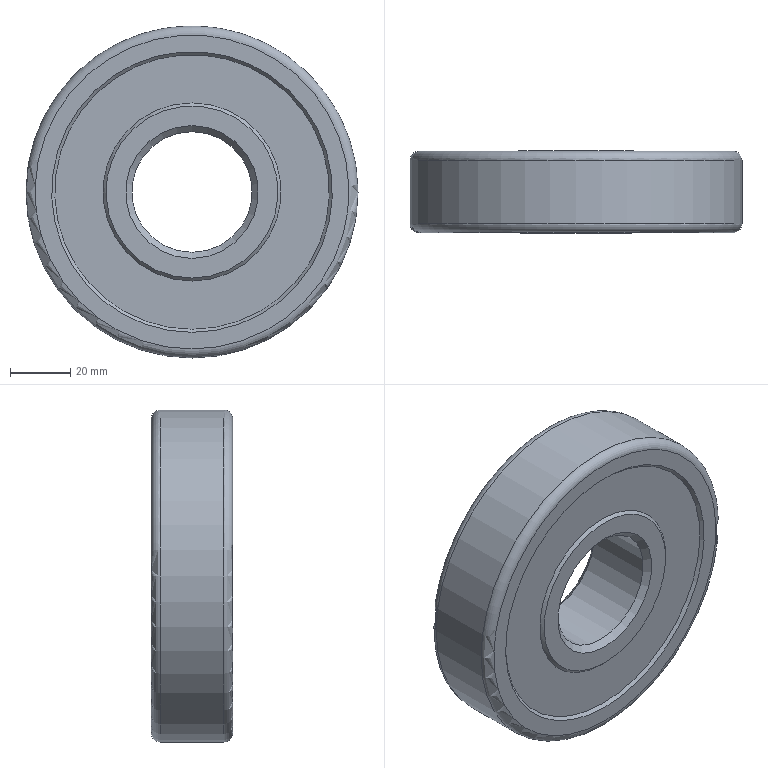Part | NX | features BREP 1, DATUM_CSYS 1 | 1 solid | 24 faces | box 110 x 27 x 110 mm | volume 123017 mm3 | plane 8 | cone 6 | cylinder 6 | torus 4 | commonest cylinder face diameters 61 x2 89 x2 40 x1 110 x1
STEP:
#1=CARTESIAN_POINT('',(0.,638.,-22.));
#2=VERTEX_POINT('',#1);
#3=CARTESIAN_POINT('',(0.,638.,0.));
#4=DIRECTION('',(0.,-1.,0.));
#5=DIRECTION('',(0.,0.,-1.));
#6=AXIS2_PLACEMENT_3D('',#3,#4,#5);
#7=CIRCLE('',#6,22.);
#8=EDGE_CURVE('',#2,#2,#7,.F.);
#9=ORIENTED_EDGE('',*,*,#8,.T.);
#10=EDGE_LOOP('',(#9));
#11=FACE_BOUND('',#10,.T.);
#12=CARTESIAN_POINT('',(0.,636.,-20.));
#13=VERTEX_POINT('',#12);
#14=CARTESIAN_POINT('',(0.,636.,0.));
#15=DIRECTION('',(0.,-1.,0.));
#16=DIRECTION('',(0.,0.,-1.));
#17=AXIS2_PLACEMENT_3D('',#14,#15,#16);
#18=CIRCLE('',#17,20.);
#19=EDGE_CURVE('',#13,#13,#18,.F.);
#20=ORIENTED_EDGE('',*,*,#19,.F.);
#21=EDGE_LOOP('',(#20));
#22=FACE_BOUND('',#21,.T.);
#23=CARTESIAN_POINT('',(0.,636.,0.));
#24=DIRECTION('',(0.,1.,0.));
#25=DIRECTION('',(0.,0.,-1.));
#26=AXIS2_PLACEMENT_3D('',#23,#24,#25);
#27=CONICAL_SURFACE('',#26,20.,0.7854);
#28=ADVANCED_FACE('',(#11,#22),#27,.F.);
#29=CARTESIAN_POINT('',(0.,638.,-28.5));
#30=VERTEX_POINT('',#29);
#31=CARTESIAN_POINT('',(0.,638.,0.));
#32=DIRECTION('',(0.,-1.,0.));
#33=DIRECTION('',(0.,0.,-1.));
#34=AXIS2_PLACEMENT_3D('',#31,#32,#33);
#35=CIRCLE('',#34,28.5);
#36=EDGE_CURVE('',#30,#30,#35,.F.);
#37=ORIENTED_EDGE('',*,*,#36,.T.);
#38=EDGE_LOOP('',(#37));
#39=FACE_BOUND('',#38,.T.);
#40=ORIENTED_EDGE('',*,*,#8,.F.);
#41=EDGE_LOOP('',(#40));
#42=FACE_BOUND('',#41,.T.);
#43=CARTESIAN_POINT('',(22.,638.,0.));
#44=DIRECTION('',(0.,1.,0.));
#45=DIRECTION('',(0.,0.,-1.));
#46=AXIS2_PLACEMENT_3D('',#43,#44,#45);
#47=PLANE('',#46);
#48=ADVANCED_FACE('',(#39,#42),#47,.T.);
#49=CARTESIAN_POINT('',(0.,637.,-29.5));
#50=VERTEX_POINT('',#49);
#51=CARTESIAN_POINT('',(0.,637.,0.));
#52=DIRECTION('',(0.,-1.,0.));
#53=DIRECTION('',(0.,0.,-1.));
#54=AXIS2_PLACEMENT_3D('',#51,#52,#53);
#55=CIRCLE('',#54,29.5);
#56=EDGE_CURVE('',#50,#50,#55,.F.);
#57=ORIENTED_EDGE('',*,*,#56,.T.);
#58=EDGE_LOOP('',(#57));
#59=FACE_BOUND('',#58,.T.);
#60=ORIENTED_EDGE('',*,*,#36,.F.);
#61=EDGE_LOOP('',(#60));
#62=FACE_BOUND('',#61,.T.);
#63=CARTESIAN_POINT('',(0.,638.,0.));
#64=DIRECTION('',(0.,-1.,0.));
#65=DIRECTION('',(0.,0.,1.));
#66=AXIS2_PLACEMENT_3D('',#63,#64,#65);
#67=CONICAL_SURFACE('',#66,28.5,0.7854);
#68=ADVANCED_FACE('',(#59,#62),#67,.T.);
#69=CARTESIAN_POINT('',(0.,637.,-45.5));
#70=VERTEX_POINT('',#69);
#71=CARTESIAN_POINT('',(0.,637.,0.));
#72=DIRECTION('',(0.,-1.,0.));
#73=DIRECTION('',(0.,0.,-1.));
#74=AXIS2_PLACEMENT_3D('',#71,#72,#73);
#75=CIRCLE('',#74,45.5);
#76=EDGE_CURVE('',#70,#70,#75,.F.);
#77=ORIENTED_EDGE('',*,*,#76,.T.);
#78=EDGE_LOOP('',(#77));
#79=FACE_BOUND('',#78,.T.);
#80=ORIENTED_EDGE('',*,*,#56,.F.);
#81=EDGE_LOOP('',(#80));
#82=FACE_BOUND('',#81,.T.);
#83=CARTESIAN_POINT('',(29.5,637.,0.));
#84=DIRECTION('',(0.,1.,0.));
#85=DIRECTION('',(0.,0.,-1.));
#86=AXIS2_PLACEMENT_3D('',#83,#84,#85);
#87=PLANE('',#86);
#88=ADVANCED_FACE('',(#79,#82),#87,.T.);
#89=CARTESIAN_POINT('',(0.,638.,-46.5));
#90=VERTEX_POINT('',#89);
#91=CARTESIAN_POINT('',(0.,638.,0.));
#92=DIRECTION('',(0.,-1.,0.));
#93=DIRECTION('',(0.,0.,-1.));
#94=AXIS2_PLACEMENT_3D('',#91,#92,#93);
#95=CIRCLE('',#94,46.5);
#96=EDGE_CURVE('',#90,#90,#95,.F.);
#97=ORIENTED_EDGE('',*,*,#96,.T.);
#98=EDGE_LOOP('',(#97));
#99=FACE_BOUND('',#98,.T.);
#100=ORIENTED_EDGE('',*,*,#76,.F.);
#101=EDGE_LOOP('',(#100));
#102=FACE_BOUND('',#101,.T.);
#103=CARTESIAN_POINT('',(0.,637.,0.));
#104=DIRECTION('',(0.,1.,0.));
#105=DIRECTION('',(0.,0.,-1.));
#106=AXIS2_PLACEMENT_3D('',#103,#104,#105);
#107=CONICAL_SURFACE('',#106,45.5,0.7854);
#108=ADVANCED_FACE('',(#99,#102),#107,.F.);
#109=CARTESIAN_POINT('',(0.,638.,-52.));
#110=VERTEX_POINT('',#109);
#111=CARTESIAN_POINT('',(0.,638.,0.));
#112=DIRECTION('',(0.,-1.,0.));
#113=DIRECTION('',(0.,0.,-1.));
#114=AXIS2_PLACEMENT_3D('',#111,#112,#113);
#115=CIRCLE('',#114,52.);
#116=EDGE_CURVE('',#110,#110,#115,.F.);
#117=ORIENTED_EDGE('',*,*,#116,.T.);
#118=EDGE_LOOP('',(#117));
#119=FACE_BOUND('',#118,.T.);
#120=ORIENTED_EDGE('',*,*,#96,.F.);
#121=EDGE_LOOP('',(#120));
#122=FACE_BOUND('',#121,.T.);
#123=CARTESIAN_POINT('',(46.5,638.,0.));
#124=DIRECTION('',(0.,1.,0.));
#125=DIRECTION('',(0.,0.,-1.));
#126=AXIS2_PLACEMENT_3D('',#123,#124,#125);
#127=PLANE('',#126);
#128=ADVANCED_FACE('',(#119,#122),#127,.T.);
#129=CARTESIAN_POINT('',(0.,635.,-55.));
#130=VERTEX_POINT('',#129);
#131=CARTESIAN_POINT('',(0.,635.,0.));
#132=DIRECTION('',(0.,-1.,0.));
#133=DIRECTION('',(0.,0.,-1.));
#134=AXIS2_PLACEMENT_3D('',#131,#132,#133);
#135=CIRCLE('',#134,55.);
#136=EDGE_CURVE('',#130,#130,#135,.F.);
#137=ORIENTED_EDGE('',*,*,#136,.T.);
#138=EDGE_LOOP('',(#137));
#139=FACE_BOUND('',#138,.T.);
#140=ORIENTED_EDGE('',*,*,#116,.F.);
#141=EDGE_LOOP('',(#140));
#142=FACE_BOUND('',#141,.T.);
#143=CARTESIAN_POINT('',(0.,635.,0.));
#144=DIRECTION('',(0.,1.,0.));
#145=DIRECTION('',(0.,0.,-1.));
#146=AXIS2_PLACEMENT_3D('',#143,#144,#145);
#147=TOROIDAL_SURFACE('',#146,52.,3.);
#148=ADVANCED_FACE('',(#139,#142),#147,.T.);
#149=CARTESIAN_POINT('',(0.,614.,-55.));
#150=VERTEX_POINT('',#149);
#151=CARTESIAN_POINT('',(0.,614.,0.));
#152=DIRECTION('',(0.,-1.,0.));
#153=DIRECTION('',(0.,0.,-1.));
#154=AXIS2_PLACEMENT_3D('',#151,#152,#153);
#155=CIRCLE('',#154,55.);
#156=EDGE_CURVE('',#150,#150,#155,.F.);
#157=ORIENTED_EDGE('',*,*,#156,.T.);
#158=EDGE_LOOP('',(#157));
#159=FACE_BOUND('',#158,.T.);
#160=ORIENTED_EDGE('',*,*,#136,.F.);
#161=EDGE_LOOP('',(#160));
#162=FACE_BOUND('',#161,.T.);
#163=CARTESIAN_POINT('',(0.,611.,0.));
#164=DIRECTION('',(0.,1.,0.));
#165=DIRECTION('',(0.,0.,-1.));
#166=AXIS2_PLACEMENT_3D('',#163,#164,#165);
#167=CYLINDRICAL_SURFACE('',#166,55.);
#168=ADVANCED_FACE('',(#159,#162),#167,.T.);
#169=CARTESIAN_POINT('',(0.,611.,-52.));
#170=VERTEX_POINT('',#169);
#171=CARTESIAN_POINT('',(0.,611.,0.));
#172=DIRECTION('',(0.,-1.,0.));
#173=DIRECTION('',(0.,0.,-1.));
#174=AXIS2_PLACEMENT_3D('',#171,#172,#173);
#175=CIRCLE('',#174,52.);
#176=EDGE_CURVE('',#170,#170,#175,.F.);
#177=ORIENTED_EDGE('',*,*,#176,.T.);
#178=EDGE_LOOP('',(#177));
#179=FACE_BOUND('',#178,.T.);
#180=ORIENTED_EDGE('',*,*,#156,.F.);
#181=EDGE_LOOP('',(#180));
#182=FACE_BOUND('',#181,.T.);
#183=CARTESIAN_POINT('',(0.,614.,0.));
#184=DIRECTION('',(0.,1.,0.));
#185=DIRECTION('',(0.,0.,-1.));
#186=AXIS2_PLACEMENT_3D('',#183,#184,#185);
#187=TOROIDAL_SURFACE('',#186,52.,3.);
#188=ADVANCED_FACE('',(#179,#182),#187,.T.);
#189=CARTESIAN_POINT('',(0.,611.,-46.5));
#190=VERTEX_POINT('',#189);
#191=CARTESIAN_POINT('',(0.,611.,0.));
#192=DIRECTION('',(0.,-1.,0.));
#193=DIRECTION('',(0.,0.,-1.));
#194=AXIS2_PLACEMENT_3D('',#191,#192,#193);
#195=CIRCLE('',#194,46.5);
#196=EDGE_CURVE('',#190,#190,#195,.F.);
#197=ORIENTED_EDGE('',*,*,#196,.T.);
#198=EDGE_LOOP('',(#197));
#199=FACE_BOUND('',#198,.T.);
#200=ORIENTED_EDGE('',*,*,#176,.F.);
#201=EDGE_LOOP('',(#200));
#202=FACE_BOUND('',#201,.T.);
#203=CARTESIAN_POINT('',(52.,611.,0.));
#204=DIRECTION('',(0.,-1.,0.));
#205=DIRECTION('',(0.,0.,1.));
#206=AXIS2_PLACEMENT_3D('',#203,#204,#205);
#207=PLANE('',#206);
#208=ADVANCED_FACE('',(#199,#202),#207,.T.);
#209=CARTESIAN_POINT('',(0.,612.,-45.5));
#210=VERTEX_POINT('',#209);
#211=CARTESIAN_POINT('',(0.,612.,0.));
#212=DIRECTION('',(0.,-1.,0.));
#213=DIRECTION('',(0.,0.,-1.));
#214=AXIS2_PLACEMENT_3D('',#211,#212,#213);
#215=CIRCLE('',#214,45.5);
#216=EDGE_CURVE('',#210,#210,#215,.F.);
#217=ORIENTED_EDGE('',*,*,#216,.T.);
#218=EDGE_LOOP('',(#217));
#219=FACE_BOUND('',#218,.T.);
#220=ORIENTED_EDGE('',*,*,#196,.F.);
#221=EDGE_LOOP('',(#220));
#222=FACE_BOUND('',#221,.T.);
#223=CARTESIAN_POINT('',(0.,611.,0.));
#224=DIRECTION('',(0.,-1.,0.));
#225=DIRECTION('',(0.,0.,1.));
#226=AXIS2_PLACEMENT_3D('',#223,#224,#225);
#227=CONICAL_SURFACE('',#226,46.5,0.7854);
#228=ADVANCED_FACE('',(#219,#222),#227,.F.);
#229=CARTESIAN_POINT('',(0.,612.,-29.5));
#230=VERTEX_POINT('',#229);
#231=CARTESIAN_POINT('',(0.,612.,0.));
#232=DIRECTION('',(0.,-1.,0.));
#233=DIRECTION('',(0.,0.,-1.));
#234=AXIS2_PLACEMENT_3D('',#231,#232,#233);
#235=CIRCLE('',#234,29.5);
#236=EDGE_CURVE('',#230,#230,#235,.F.);
#237=ORIENTED_EDGE('',*,*,#236,.T.);
#238=EDGE_LOOP('',(#237));
#239=FACE_BOUND('',#238,.T.);
#240=ORIENTED_EDGE('',*,*,#216,.F.);
#241=EDGE_LOOP('',(#240));
#242=FACE_BOUND('',#241,.T.);
#243=CARTESIAN_POINT('',(45.5,612.,0.));
#244=DIRECTION('',(0.,-1.,0.));
#245=DIRECTION('',(0.,0.,1.));
#246=AXIS2_PLACEMENT_3D('',#243,#244,#245);
#247=PLANE('',#246);
#248=ADVANCED_FACE('',(#239,#242),#247,.T.);
#249=CARTESIAN_POINT('',(0.,611.,-28.5));
#250=VERTEX_POINT('',#249);
#251=CARTESIAN_POINT('',(0.,611.,0.));
#252=DIRECTION('',(0.,-1.,0.));
#253=DIRECTION('',(0.,0.,-1.));
#254=AXIS2_PLACEMENT_3D('',#251,#252,#253);
#255=CIRCLE('',#254,28.5);
#256=EDGE_CURVE('',#250,#250,#255,.F.);
#257=ORIENTED_EDGE('',*,*,#256,.T.);
#258=EDGE_LOOP('',(#257));
#259=FACE_BOUND('',#258,.T.);
#260=ORIENTED_EDGE('',*,*,#236,.F.);
#261=EDGE_LOOP('',(#260));
#262=FACE_BOUND('',#261,.T.);
#263=CARTESIAN_POINT('',(0.,612.,0.));
#264=DIRECTION('',(0.,1.,0.));
#265=DIRECTION('',(0.,0.,-1.));
#266=AXIS2_PLACEMENT_3D('',#263,#264,#265);
#267=CONICAL_SURFACE('',#266,29.5,0.7854);
#268=ADVANCED_FACE('',(#259,#262),#267,.T.);
#269=CARTESIAN_POINT('',(0.,611.,-22.));
#270=VERTEX_POINT('',#269);
#271=CARTESIAN_POINT('',(0.,611.,0.));
#272=DIRECTION('',(0.,-1.,0.));
#273=DIRECTION('',(0.,0.,-1.));
#274=AXIS2_PLACEMENT_3D('',#271,#272,#273);
#275=CIRCLE('',#274,22.);
#276=EDGE_CURVE('',#270,#270,#275,.F.);
#277=ORIENTED_EDGE('',*,*,#276,.T.);
#278=EDGE_LOOP('',(#277));
#279=FACE_BOUND('',#278,.T.);
#280=ORIENTED_EDGE('',*,*,#256,.F.);
#281=EDGE_LOOP('',(#280));
#282=FACE_BOUND('',#281,.T.);
#283=CARTESIAN_POINT('',(28.5,611.,0.));
#284=DIRECTION('',(0.,-1.,0.));
#285=DIRECTION('',(0.,0.,1.));
#286=AXIS2_PLACEMENT_3D('',#283,#284,#285);
#287=PLANE('',#286);
#288=ADVANCED_FACE('',(#279,#282),#287,.T.);
#289=CARTESIAN_POINT('',(0.,613.,-20.));
#290=VERTEX_POINT('',#289);
#291=CARTESIAN_POINT('',(0.,613.,0.));
#292=DIRECTION('',(0.,-1.,0.));
#293=DIRECTION('',(0.,0.,-1.));
#294=AXIS2_PLACEMENT_3D('',#291,#292,#293);
#295=CIRCLE('',#294,20.);
#296=EDGE_CURVE('',#290,#290,#295,.F.);
#297=ORIENTED_EDGE('',*,*,#296,.T.);
#298=EDGE_LOOP('',(#297));
#299=FACE_BOUND('',#298,.T.);
#300=ORIENTED_EDGE('',*,*,#276,.F.);
#301=EDGE_LOOP('',(#300));
#302=FACE_BOUND('',#301,.T.);
#303=CARTESIAN_POINT('',(0.,611.,0.));
#304=DIRECTION('',(0.,-1.,0.));
#305=DIRECTION('',(0.,0.,1.));
#306=AXIS2_PLACEMENT_3D('',#303,#304,#305);
#307=CONICAL_SURFACE('',#306,22.,0.7854);
#308=ADVANCED_FACE('',(#299,#302),#307,.F.);
#309=ORIENTED_EDGE('',*,*,#19,.T.);
#310=EDGE_LOOP('',(#309));
#311=FACE_BOUND('',#310,.T.);
#312=ORIENTED_EDGE('',*,*,#296,.F.);
#313=EDGE_LOOP('',(#312));
#314=FACE_BOUND('',#313,.T.);
#315=CARTESIAN_POINT('',(0.,611.,0.));
#316=DIRECTION('',(0.,1.,0.));
#317=DIRECTION('',(0.,0.,-1.));
#318=AXIS2_PLACEMENT_3D('',#315,#316,#317);
#319=CYLINDRICAL_SURFACE('',#318,20.);
#320=ADVANCED_FACE('',(#311,#314),#319,.F.);
#321=CLOSED_SHELL('',(#28,#48,#68,#88,#108,#128,#148,#168,#188,#208,#228,#248,#268,#288,#308,#320));
#322=CARTESIAN_POINT('',(0.,617.359,-30.5));
#323=VERTEX_POINT('',#322);
#324=CARTESIAN_POINT('',(0.,617.359,0.));
#325=DIRECTION('',(0.,-1.,0.));
#326=DIRECTION('',(0.,0.,-1.));
#327=AXIS2_PLACEMENT_3D('',#324,#325,#326);
#328=CIRCLE('',#327,30.5);
#329=EDGE_CURVE('',#323,#323,#328,.F.);
#330=ORIENTED_EDGE('',*,*,#329,.T.);
#331=EDGE_LOOP('',(#330));
#332=FACE_BOUND('',#331,.T.);
#333=CARTESIAN_POINT('',(0.,631.641,-30.5));
#334=VERTEX_POINT('',#333);
#335=CARTESIAN_POINT('',(0.,631.641,0.));
#336=DIRECTION('',(0.,-1.,0.));
#337=DIRECTION('',(0.,0.,-1.));
#338=AXIS2_PLACEMENT_3D('',#335,#336,#337);
#339=CIRCLE('',#338,30.5);
#340=EDGE_CURVE('',#334,#334,#339,.F.);
#341=ORIENTED_EDGE('',*,*,#340,.F.);
#342=EDGE_LOOP('',(#341));
#343=FACE_BOUND('',#342,.T.);
#344=CARTESIAN_POINT('',(0.,624.5,0.));
#345=DIRECTION('',(0.,1.,0.));
#346=DIRECTION('',(0.,0.,-1.));
#347=AXIS2_PLACEMENT_3D('',#344,#345,#346);
#348=TOROIDAL_SURFACE('',#347,37.5,10.);
#349=ADVANCED_FACE('',(#332,#343),#348,.F.);
#350=CARTESIAN_POINT('',(0.,613.,-30.5));
#351=VERTEX_POINT('',#350);
#352=CARTESIAN_POINT('',(0.,613.,0.));
#353=DIRECTION('',(0.,-1.,0.));
#354=DIRECTION('',(0.,0.,-1.));
#355=AXIS2_PLACEMENT_3D('',#352,#353,#354);
#356=CIRCLE('',#355,30.5);
#357=EDGE_CURVE('',#351,#351,#356,.F.);
#358=ORIENTED_EDGE('',*,*,#357,.T.);
#359=EDGE_LOOP('',(#358));
#360=FACE_BOUND('',#359,.T.);
#361=ORIENTED_EDGE('',*,*,#329,.F.);
#362=EDGE_LOOP('',(#361));
#363=FACE_BOUND('',#362,.T.);
#364=CARTESIAN_POINT('',(0.,611.,0.));
#365=DIRECTION('',(0.,1.,0.));
#366=DIRECTION('',(0.,0.,-1.));
#367=AXIS2_PLACEMENT_3D('',#364,#365,#366);
#368=CYLINDRICAL_SURFACE('',#367,30.5);
#369=ADVANCED_FACE('',(#360,#363),#368,.T.);
#370=CARTESIAN_POINT('',(0.,613.,-44.5));
#371=VERTEX_POINT('',#370);
#372=CARTESIAN_POINT('',(0.,613.,0.));
#373=DIRECTION('',(0.,-1.,0.));
#374=DIRECTION('',(0.,0.,-1.));
#375=AXIS2_PLACEMENT_3D('',#372,#373,#374);
#376=CIRCLE('',#375,44.5);
#377=EDGE_CURVE('',#371,#371,#376,.F.);
#378=ORIENTED_EDGE('',*,*,#377,.T.);
#379=EDGE_LOOP('',(#378));
#380=FACE_BOUND('',#379,.T.);
#381=ORIENTED_EDGE('',*,*,#357,.F.);
#382=EDGE_LOOP('',(#381));
#383=FACE_BOUND('',#382,.T.);
#384=CARTESIAN_POINT('',(30.5,613.,0.));
#385=DIRECTION('',(0.,1.,0.));
#386=DIRECTION('',(0.,0.,-1.));
#387=AXIS2_PLACEMENT_3D('',#384,#385,#386);
#388=PLANE('',#387);
#389=ADVANCED_FACE('',(#380,#383),#388,.T.);
#390=CARTESIAN_POINT('',(0.,617.359,-44.5));
#391=VERTEX_POINT('',#390);
#392=CARTESIAN_POINT('',(0.,617.359,0.));
#393=DIRECTION('',(0.,-1.,0.));
#394=DIRECTION('',(0.,0.,-1.));
#395=AXIS2_PLACEMENT_3D('',#392,#393,#394);
#396=CIRCLE('',#395,44.5);
#397=EDGE_CURVE('',#391,#391,#396,.F.);
#398=ORIENTED_EDGE('',*,*,#397,.T.);
#399=EDGE_LOOP('',(#398));
#400=FACE_BOUND('',#399,.T.);
#401=ORIENTED_EDGE('',*,*,#377,.F.);
#402=EDGE_LOOP('',(#401));
#403=FACE_BOUND('',#402,.T.);
#404=CARTESIAN_POINT('',(0.,611.,0.));
#405=DIRECTION('',(0.,1.,0.));
#406=DIRECTION('',(0.,0.,-1.));
#407=AXIS2_PLACEMENT_3D('',#404,#405,#406);
#408=CYLINDRICAL_SURFACE('',#407,44.5);
#409=ADVANCED_FACE('',(#400,#403),#408,.F.);
#410=CARTESIAN_POINT('',(0.,631.641,-44.5));
#411=VERTEX_POINT('',#410);
#412=CARTESIAN_POINT('',(0.,631.641,0.));
#413=DIRECTION('',(0.,-1.,0.));
#414=DIRECTION('',(0.,0.,-1.));
#415=AXIS2_PLACEMENT_3D('',#412,#413,#414);
#416=CIRCLE('',#415,44.5);
#417=EDGE_CURVE('',#411,#411,#416,.F.);
#418=ORIENTED_EDGE('',*,*,#417,.T.);
#419=EDGE_LOOP('',(#418));
#420=FACE_BOUND('',#419,.T.);
#421=ORIENTED_EDGE('',*,*,#397,.F.);
#422=EDGE_LOOP('',(#421));
#423=FACE_BOUND('',#422,.T.);
#424=CARTESIAN_POINT('',(0.,624.5,0.));
#425=DIRECTION('',(0.,1.,0.));
#426=DIRECTION('',(0.,0.,-1.));
#427=AXIS2_PLACEMENT_3D('',#424,#425,#426);
#428=TOROIDAL_SURFACE('',#427,37.5,10.);
#429=ADVANCED_FACE('',(#420,#423),#428,.F.);
#430=CARTESIAN_POINT('',(0.,636.,-44.5));
#431=VERTEX_POINT('',#430);
#432=CARTESIAN_POINT('',(0.,636.,0.));
#433=DIRECTION('',(0.,-1.,0.));
#434=DIRECTION('',(0.,0.,-1.));
#435=AXIS2_PLACEMENT_3D('',#432,#433,#434);
#436=CIRCLE('',#435,44.5);
#437=EDGE_CURVE('',#431,#431,#436,.F.);
#438=ORIENTED_EDGE('',*,*,#437,.T.);
#439=EDGE_LOOP('',(#438));
#440=FACE_BOUND('',#439,.T.);
#441=ORIENTED_EDGE('',*,*,#417,.F.);
#442=EDGE_LOOP('',(#441));
#443=FACE_BOUND('',#442,.T.);
#444=CARTESIAN_POINT('',(0.,611.,0.));
#445=DIRECTION('',(0.,1.,0.));
#446=DIRECTION('',(0.,0.,-1.));
#447=AXIS2_PLACEMENT_3D('',#444,#445,#446);
#448=CYLINDRICAL_SURFACE('',#447,44.5);
#449=ADVANCED_FACE('',(#440,#443),#448,.F.);
#450=CARTESIAN_POINT('',(0.,636.,-30.5));
#451=VERTEX_POINT('',#450);
#452=CARTESIAN_POINT('',(0.,636.,0.));
#453=DIRECTION('',(0.,-1.,0.));
#454=DIRECTION('',(0.,0.,-1.));
#455=AXIS2_PLACEMENT_3D('',#452,#453,#454);
#456=CIRCLE('',#455,30.5);
#457=EDGE_CURVE('',#451,#451,#456,.F.);
#458=ORIENTED_EDGE('',*,*,#457,.T.);
#459=EDGE_LOOP('',(#458));
#460=FACE_BOUND('',#459,.T.);
#461=ORIENTED_EDGE('',*,*,#437,.F.);
#462=EDGE_LOOP('',(#461));
#463=FACE_BOUND('',#462,.T.);
#464=CARTESIAN_POINT('',(44.5,636.,0.));
#465=DIRECTION('',(0.,-1.,0.));
#466=DIRECTION('',(0.,0.,1.));
#467=AXIS2_PLACEMENT_3D('',#464,#465,#466);
#468=PLANE('',#467);
#469=ADVANCED_FACE('',(#460,#463),#468,.T.);
#470=ORIENTED_EDGE('',*,*,#340,.T.);
#471=EDGE_LOOP('',(#470));
#472=FACE_BOUND('',#471,.T.);
#473=ORIENTED_EDGE('',*,*,#457,.F.);
#474=EDGE_LOOP('',(#473));
#475=FACE_BOUND('',#474,.T.);
#476=CARTESIAN_POINT('',(0.,611.,0.));
#477=DIRECTION('',(0.,1.,0.));
#478=DIRECTION('',(0.,0.,-1.));
#479=AXIS2_PLACEMENT_3D('',#476,#477,#478);
#480=CYLINDRICAL_SURFACE('',#479,30.5);
#481=ADVANCED_FACE('',(#472,#475),#480,.T.);
#482=CLOSED_SHELL('',(#349,#369,#389,#409,#429,#449,#469,#481));
#483=ORIENTED_CLOSED_SHELL('',*,#482,.F.);
#484=BREP_WITH_VOIDS('',#321,(#483));
#485=(LENGTH_UNIT()NAMED_UNIT(*)SI_UNIT(.MILLI.,.METRE.));
#486=UNCERTAINTY_MEASURE_WITH_UNIT(LENGTH_MEASURE(0.00001),#485,'','');
#487=(NAMED_UNIT(*)PLANE_ANGLE_UNIT()SI_UNIT($,.RADIAN.));
#488=(NAMED_UNIT(*)SI_UNIT($,.STERADIAN.)SOLID_ANGLE_UNIT());
#489=(GEOMETRIC_REPRESENTATION_CONTEXT(3)GLOBAL_UNCERTAINTY_ASSIGNED_CONTEXT((#486))GLOBAL_UNIT_ASSIGNED_CONTEXT((#485,#487,#488))REPRESENTATION_CONTEXT('',''));
#490=ADVANCED_BREP_SHAPE_REPRESENTATION('',(#484),#489);